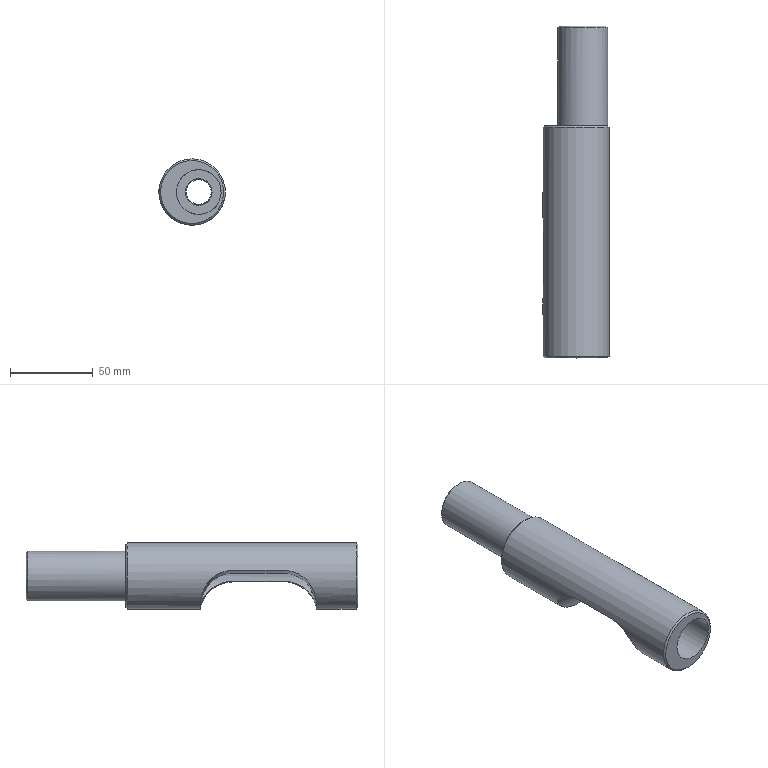Part | NX | features DATUM_CSYS 8, EXTRUDE 8, SKETCH 7, CHAMFER 2 | 1 solid | 19 faces | box 40 x 200 x 40 mm | volume 117689 mm3 | cylinder 8 | plane 8 | cone 3 | commonest cylinder face diameters 40 x3 15 x1 16 x1 27 x1 27.5 x1 30 x1
STEP:
#1=CARTESIAN_POINT('',(12.,40.,0.));
#2=VERTEX_POINT('',#1);
#3=CARTESIAN_POINT('',(4.,40.,0.));
#4=DIRECTION('',(0.,1.,0.));
#5=DIRECTION('',(1.,0.,0.));
#6=AXIS2_PLACEMENT_3D('',#3,#4,#5);
#7=CIRCLE('',#6,8.);
#8=EDGE_CURVE('',#2,#2,#7,.F.);
#9=ORIENTED_EDGE('',*,*,#8,.F.);
#10=EDGE_LOOP('',(#9));
#11=FACE_BOUND('',#10,.T.);
#12=CARTESIAN_POINT('',(4.,-40.,-8.));
#13=VERTEX_POINT('',#12);
#14=CARTESIAN_POINT('',(4.,-40.,0.));
#15=DIRECTION('',(0.,-1.,0.));
#16=DIRECTION('',(0.,0.,-1.));
#17=AXIS2_PLACEMENT_3D('',#14,#15,#16);
#18=CIRCLE('',#17,8.);
#19=EDGE_CURVE('',#13,#13,#18,.F.);
#20=ORIENTED_EDGE('',*,*,#19,.F.);
#21=EDGE_LOOP('',(#20));
#22=FACE_BOUND('',#21,.T.);
#23=CARTESIAN_POINT('',(4.,-192.,0.));
#24=DIRECTION('',(0.,1.,0.));
#25=DIRECTION('',(0.,0.,1.));
#26=AXIS2_PLACEMENT_3D('',#23,#24,#25);
#27=CYLINDRICAL_SURFACE('',#26,8.);
#28=ADVANCED_FACE('',(#11,#22),#27,.F.);
#29=CARTESIAN_POINT('',(0.,-139.,-20.));
#30=VERTEX_POINT('',#29);
#31=CARTESIAN_POINT('',(0.,-139.,0.));
#32=DIRECTION('',(0.,-1.,0.));
#33=DIRECTION('',(0.,0.,-1.));
#34=AXIS2_PLACEMENT_3D('',#31,#32,#33);
#35=CIRCLE('',#34,20.);
#36=EDGE_CURVE('',#30,#30,#35,.F.);
#37=ORIENTED_EDGE('',*,*,#36,.T.);
#38=EDGE_LOOP('',(#37));
#39=FACE_BOUND('',#38,.T.);
#40=CARTESIAN_POINT('',(-19.696,-65.,3.473));
#41=VERTEX_POINT('',#40);
#42=CARTESIAN_POINT('',(-19.696,-95.,3.473));
#43=VERTEX_POINT('',#42);
#44=CARTESIAN_POINT('',(-19.696,-140.,3.473));
#45=DIRECTION('',(0.,1.,0.));
#46=VECTOR('',#45,1000.);
#47=LINE('',#44,#46);
#48=EDGE_CURVE('',#41,#43,#47,.F.);
#49=ORIENTED_EDGE('',*,*,#48,.T.);
#50=CARTESIAN_POINT('',(19.696,-95.,-3.473));
#51=VERTEX_POINT('',#50);
#52=CARTESIAN_POINT('',(-19.696,-95.,3.473));
#53=CARTESIAN_POINT('',(-19.696,-96.79,3.473));
#54=CARTESIAN_POINT('',(-19.786,-100.303,3.009));
#55=CARTESIAN_POINT('',(-20.039,-105.264,0.9372));
#56=CARTESIAN_POINT('',(-19.981,-109.466,-2.426));
#57=CARTESIAN_POINT('',(-19.027,-112.527,-6.766));
#58=CARTESIAN_POINT('',(-16.741,-114.246,-11.36));
#59=CARTESIAN_POINT('',(-11.982,-115.102,-16.706));
#60=CARTESIAN_POINT('',(-3.665,-114.932,-20.648));
#61=CARTESIAN_POINT('',(5.488,-115.101,-19.81));
#62=CARTESIAN_POINT('',(11.786,-114.26,-16.443));
#63=CARTESIAN_POINT('',(15.516,-112.566,-12.928));
#64=CARTESIAN_POINT('',(17.927,-109.514,-9.156));
#65=CARTESIAN_POINT('',(19.146,-105.3,-5.992));
#66=CARTESIAN_POINT('',(19.622,-100.328,-3.944));
#67=CARTESIAN_POINT('',(19.696,-96.794,-3.473));
#68=CARTESIAN_POINT('',(19.696,-95.,-3.473));
#69=B_SPLINE_CURVE_WITH_KNOTS('',3,(#52,#53,#54,#55,#56,#57,#58,#59,#60,#61,#62,#63,#64,#65,#66,#67,#68),.UNSPECIFIED.,.F.,.F.,(4,1,1,1,1,1,1,1,1,1,1,1,1,1,4),(0.,0.005295,0.01059,0.01589,0.02118,0.02648,0.03177,0.04236,0.05295,0.05825,0.06354,0.06884,0.07413,0.07943,0.08472),.UNSPECIFIED.);
#70=EDGE_CURVE('',#43,#51,#69,.T.);
#71=ORIENTED_EDGE('',*,*,#70,.T.);
#72=CARTESIAN_POINT('',(19.696,-65.,-3.473));
#73=VERTEX_POINT('',#72);
#74=CARTESIAN_POINT('',(19.696,-140.,-3.473));
#75=DIRECTION('',(0.,1.,0.));
#76=VECTOR('',#75,1000.);
#77=LINE('',#74,#76);
#78=EDGE_CURVE('',#51,#73,#77,.T.);
#79=ORIENTED_EDGE('',*,*,#78,.T.);
#80=CARTESIAN_POINT('',(19.696,-65.,-3.473));
#81=CARTESIAN_POINT('',(19.696,-63.21,-3.473));
#82=CARTESIAN_POINT('',(19.622,-59.697,-3.94));
#83=CARTESIAN_POINT('',(19.151,-54.736,-5.973));
#84=CARTESIAN_POINT('',(17.946,-50.534,-9.114));
#85=CARTESIAN_POINT('',(15.566,-47.473,-12.866));
#86=CARTESIAN_POINT('',(11.846,-45.754,-16.401));
#87=CARTESIAN_POINT('',(5.545,-44.898,-19.797));
#88=CARTESIAN_POINT('',(-3.618,-45.068,-20.656));
#89=CARTESIAN_POINT('',(-11.933,-44.899,-16.738));
#90=CARTESIAN_POINT('',(-16.699,-45.74,-11.42));
#91=CARTESIAN_POINT('',(-19.002,-47.434,-6.841));
#92=CARTESIAN_POINT('',(-19.978,-50.486,-2.473));
#93=CARTESIAN_POINT('',(-20.04,-54.7,0.9177));
#94=CARTESIAN_POINT('',(-19.787,-59.672,3.005));
#95=CARTESIAN_POINT('',(-19.696,-63.206,3.473));
#96=CARTESIAN_POINT('',(-19.696,-65.,3.473));
#97=B_SPLINE_CURVE_WITH_KNOTS('',3,(#80,#81,#82,#83,#84,#85,#86,#87,#88,#89,#90,#91,#92,#93,#94,#95,#96),.UNSPECIFIED.,.F.,.F.,(4,1,1,1,1,1,1,1,1,1,1,1,1,1,4),(0.,0.005295,0.01059,0.01589,0.02118,0.02648,0.03177,0.04236,0.05295,0.05825,0.06354,0.06884,0.07413,0.07943,0.08472),.UNSPECIFIED.);
#98=EDGE_CURVE('',#73,#41,#97,.T.);
#99=ORIENTED_EDGE('',*,*,#98,.T.);
#100=EDGE_LOOP('',(#49,#71,#79,#99));
#101=FACE_BOUND('',#100,.T.);
#102=CARTESIAN_POINT('',(0.,-1.,-20.));
#103=VERTEX_POINT('',#102);
#104=CARTESIAN_POINT('',(0.,-1.,0.));
#105=DIRECTION('',(0.,-1.,0.));
#106=DIRECTION('',(0.,0.,-1.));
#107=AXIS2_PLACEMENT_3D('',#104,#105,#106);
#108=CIRCLE('',#107,20.);
#109=EDGE_CURVE('',#103,#103,#108,.T.);
#110=ORIENTED_EDGE('',*,*,#109,.T.);
#111=EDGE_LOOP('',(#110));
#112=FACE_BOUND('',#111,.T.);
#113=CARTESIAN_POINT('',(0.,-140.,0.));
#114=DIRECTION('',(0.,1.,0.));
#115=DIRECTION('',(0.,0.,1.));
#116=AXIS2_PLACEMENT_3D('',#113,#114,#115);
#117=CYLINDRICAL_SURFACE('',#116,20.);
#118=ADVANCED_FACE('',(#39,#101,#112),#117,.T.);
#119=CARTESIAN_POINT('',(0.,-140.,-19.));
#120=VERTEX_POINT('',#119);
#121=CARTESIAN_POINT('',(0.,-140.,0.));
#122=DIRECTION('',(0.,-1.,0.));
#123=DIRECTION('',(0.,0.,-1.));
#124=AXIS2_PLACEMENT_3D('',#121,#122,#123);
#125=CIRCLE('',#124,19.);
#126=EDGE_CURVE('',#120,#120,#125,.T.);
#127=ORIENTED_EDGE('',*,*,#126,.T.);
#128=EDGE_LOOP('',(#127));
#129=FACE_BOUND('',#128,.T.);
#130=CARTESIAN_POINT('',(17.5,-140.,0.));
#131=VERTEX_POINT('',#130);
#132=CARTESIAN_POINT('',(4.,-140.,0.));
#133=DIRECTION('',(0.,-1.,0.));
#134=DIRECTION('',(1.,0.,0.));
#135=AXIS2_PLACEMENT_3D('',#132,#133,#134);
#136=CIRCLE('',#135,13.5);
#137=EDGE_CURVE('',#131,#131,#136,.T.);
#138=ORIENTED_EDGE('',*,*,#137,.F.);
#139=EDGE_LOOP('',(#138));
#140=FACE_BOUND('',#139,.T.);
#141=CARTESIAN_POINT('',(0.,-140.,0.));
#142=DIRECTION('',(0.,-1.,0.));
#143=DIRECTION('',(0.,0.,-1.));
#144=AXIS2_PLACEMENT_3D('',#141,#142,#143);
#145=PLANE('',#144);
#146=ADVANCED_FACE('',(#129,#140),#145,.T.);
#147=CARTESIAN_POINT('',(19.,0.,0.));
#148=VERTEX_POINT('',#147);
#149=CARTESIAN_POINT('',(4.,0.,0.));
#150=DIRECTION('',(0.,1.,0.));
#151=DIRECTION('',(1.,0.,0.));
#152=AXIS2_PLACEMENT_3D('',#149,#150,#151);
#153=CIRCLE('',#152,15.);
#154=EDGE_CURVE('',#148,#148,#153,.T.);
#155=ORIENTED_EDGE('',*,*,#154,.F.);
#156=CARTESIAN_POINT('',(0.,0.,0.));
#157=DIRECTION('',(0.,-1.,0.));
#158=DIRECTION('',(0.,0.,-1.));
#159=AXIS2_PLACEMENT_3D('',#156,#157,#158);
#160=CIRCLE('',#159,19.);
#161=EDGE_CURVE('',#148,#148,#160,.F.);
#162=ORIENTED_EDGE('',*,*,#161,.T.);
#163=EDGE_LOOP('',(#155,#162));
#164=FACE_BOUND('',#163,.T.);
#165=CARTESIAN_POINT('',(0.,0.,0.));
#166=DIRECTION('',(0.,-1.,0.));
#167=DIRECTION('',(0.,0.,-1.));
#168=AXIS2_PLACEMENT_3D('',#165,#166,#167);
#169=PLANE('',#168);
#170=ADVANCED_FACE('',(#164),#169,.F.);
#171=CARTESIAN_POINT('',(4.,59.,15.));
#172=VERTEX_POINT('',#171);
#173=CARTESIAN_POINT('',(4.,59.,0.));
#174=DIRECTION('',(0.,1.,0.));
#175=DIRECTION('',(0.,0.,1.));
#176=AXIS2_PLACEMENT_3D('',#173,#174,#175);
#177=CIRCLE('',#176,15.);
#178=EDGE_CURVE('',#172,#172,#177,.F.);
#179=ORIENTED_EDGE('',*,*,#178,.T.);
#180=EDGE_LOOP('',(#179));
#181=FACE_BOUND('',#180,.T.);
#182=ORIENTED_EDGE('',*,*,#154,.T.);
#183=EDGE_LOOP('',(#182));
#184=FACE_BOUND('',#183,.T.);
#185=CARTESIAN_POINT('',(4.,60.,0.));
#186=DIRECTION('',(0.,-1.,0.));
#187=DIRECTION('',(0.,0.,-1.));
#188=AXIS2_PLACEMENT_3D('',#185,#186,#187);
#189=CYLINDRICAL_SURFACE('',#188,15.);
#190=ADVANCED_FACE('',(#181,#184),#189,.T.);
#191=CARTESIAN_POINT('',(4.,60.,14.));
#192=VERTEX_POINT('',#191);
#193=CARTESIAN_POINT('',(4.,60.,0.));
#194=DIRECTION('',(0.,1.,0.));
#195=DIRECTION('',(0.,0.,1.));
#196=AXIS2_PLACEMENT_3D('',#193,#194,#195);
#197=CIRCLE('',#196,14.);
#198=EDGE_CURVE('',#192,#192,#197,.T.);
#199=ORIENTED_EDGE('',*,*,#198,.T.);
#200=EDGE_LOOP('',(#199));
#201=FACE_BOUND('',#200,.T.);
#202=CARTESIAN_POINT('',(11.5,60.,0.));
#203=VERTEX_POINT('',#202);
#204=CARTESIAN_POINT('',(4.,60.,0.));
#205=DIRECTION('',(0.,1.,0.));
#206=DIRECTION('',(1.,0.,0.));
#207=AXIS2_PLACEMENT_3D('',#204,#205,#206);
#208=CIRCLE('',#207,7.5);
#209=EDGE_CURVE('',#203,#203,#208,.T.);
#210=ORIENTED_EDGE('',*,*,#209,.F.);
#211=EDGE_LOOP('',(#210));
#212=FACE_BOUND('',#211,.T.);
#213=CARTESIAN_POINT('',(4.,60.,0.));
#214=DIRECTION('',(0.,1.,0.));
#215=DIRECTION('',(0.,0.,1.));
#216=AXIS2_PLACEMENT_3D('',#213,#214,#215);
#217=PLANE('',#216);
#218=ADVANCED_FACE('',(#201,#212),#217,.T.);
#219=CARTESIAN_POINT('',(11.5,40.,0.));
#220=VERTEX_POINT('',#219);
#221=CARTESIAN_POINT('',(4.,40.,0.));
#222=DIRECTION('',(0.,1.,0.));
#223=DIRECTION('',(1.,0.,0.));
#224=AXIS2_PLACEMENT_3D('',#221,#222,#223);
#225=CIRCLE('',#224,7.5);
#226=EDGE_CURVE('',#220,#220,#225,.F.);
#227=ORIENTED_EDGE('',*,*,#226,.T.);
#228=EDGE_LOOP('',(#227));
#229=FACE_BOUND('',#228,.T.);
#230=ORIENTED_EDGE('',*,*,#209,.T.);
#231=EDGE_LOOP('',(#230));
#232=FACE_BOUND('',#231,.T.);
#233=CARTESIAN_POINT('',(4.,40.,0.));
#234=DIRECTION('',(0.,1.,0.));
#235=DIRECTION('',(0.,0.,1.));
#236=AXIS2_PLACEMENT_3D('',#233,#234,#235);
#237=CYLINDRICAL_SURFACE('',#236,7.5);
#238=ADVANCED_FACE('',(#229,#232),#237,.F.);
#239=ORIENTED_EDGE('',*,*,#8,.T.);
#240=EDGE_LOOP('',(#239));
#241=FACE_BOUND('',#240,.T.);
#242=ORIENTED_EDGE('',*,*,#226,.F.);
#243=EDGE_LOOP('',(#242));
#244=FACE_BOUND('',#243,.T.);
#245=CARTESIAN_POINT('',(4.,40.,0.));
#246=DIRECTION('',(0.,1.,0.));
#247=DIRECTION('',(0.,0.,1.));
#248=AXIS2_PLACEMENT_3D('',#245,#246,#247);
#249=PLANE('',#248);
#250=ADVANCED_FACE('',(#241,#244),#249,.F.);
#251=CARTESIAN_POINT('',(-6.52,-112.,-8.461));
#252=VERTEX_POINT('',#251);
#253=CARTESIAN_POINT('',(10.992,-112.,-11.548));
#254=VERTEX_POINT('',#253);
#255=CARTESIAN_POINT('',(4.,-112.,0.));
#256=DIRECTION('',(0.,-1.,0.));
#257=DIRECTION('',(1.,0.,0.));
#258=AXIS2_PLACEMENT_3D('',#255,#256,#257);
#259=CIRCLE('',#258,13.5);
#260=EDGE_CURVE('',#252,#254,#259,.F.);
#261=ORIENTED_EDGE('',*,*,#260,.T.);
#262=CARTESIAN_POINT('',(10.992,-112.,-11.548));
#263=CARTESIAN_POINT('',(9.672,-112.63,-12.348));
#264=CARTESIAN_POINT('',(6.647,-113.44,-13.545));
#265=CARTESIAN_POINT('',(1.603,-113.771,-13.599));
#266=CARTESIAN_POINT('',(-3.106,-113.442,-11.831));
#267=CARTESIAN_POINT('',(-5.553,-112.63,-9.663));
#268=CARTESIAN_POINT('',(-6.52,-112.,-8.461));
#269=B_SPLINE_CURVE_WITH_KNOTS('',3,(#262,#263,#264,#265,#266,#267,#268),.UNSPECIFIED.,.F.,.F.,(4,1,1,1,4),(0.,0.004926,0.009852,0.01478,0.0197),.UNSPECIFIED.);
#270=EDGE_CURVE('',#254,#252,#269,.T.);
#271=ORIENTED_EDGE('',*,*,#270,.T.);
#272=EDGE_LOOP('',(#261,#271));
#273=FACE_BOUND('',#272,.T.);
#274=ORIENTED_EDGE('',*,*,#137,.T.);
#275=EDGE_LOOP('',(#274));
#276=FACE_BOUND('',#275,.T.);
#277=CARTESIAN_POINT('',(4.,-112.,0.));
#278=DIRECTION('',(0.,-1.,0.));
#279=DIRECTION('',(0.,0.,-1.));
#280=AXIS2_PLACEMENT_3D('',#277,#278,#279);
#281=CYLINDRICAL_SURFACE('',#280,13.5);
#282=ADVANCED_FACE('',(#273,#276),#281,.F.);
#283=CARTESIAN_POINT('',(-6.889,-112.,-8.396));
#284=VERTEX_POINT('',#283);
#285=CARTESIAN_POINT('',(11.361,-112.,-11.614));
#286=VERTEX_POINT('',#285);
#287=CARTESIAN_POINT('',(4.,-112.,0.));
#288=DIRECTION('',(0.,-1.,0.));
#289=DIRECTION('',(1.,0.,0.));
#290=AXIS2_PLACEMENT_3D('',#287,#288,#289);
#291=CIRCLE('',#290,13.75);
#292=EDGE_CURVE('',#284,#286,#291,.F.);
#293=ORIENTED_EDGE('',*,*,#292,.T.);
#294=CARTESIAN_POINT('',(-37.54,-112.,-2.991));
#295=DIRECTION('',(0.9848,0.,-0.1736));
#296=VECTOR('',#295,1000.);
#297=LINE('',#294,#296);
#298=EDGE_CURVE('',#286,#254,#297,.F.);
#299=ORIENTED_EDGE('',*,*,#298,.T.);
#300=ORIENTED_EDGE('',*,*,#260,.F.);
#301=CARTESIAN_POINT('',(-37.54,-112.,-2.991));
#302=DIRECTION('',(0.9848,0.,-0.1736));
#303=VECTOR('',#302,1000.);
#304=LINE('',#301,#303);
#305=EDGE_CURVE('',#252,#284,#304,.F.);
#306=ORIENTED_EDGE('',*,*,#305,.T.);
#307=EDGE_LOOP('',(#293,#299,#300,#306));
#308=FACE_BOUND('',#307,.T.);
#309=CARTESIAN_POINT('',(4.,-112.,0.));
#310=DIRECTION('',(0.,-1.,0.));
#311=DIRECTION('',(0.,0.,-1.));
#312=AXIS2_PLACEMENT_3D('',#309,#310,#311);
#313=PLANE('',#312);
#314=ADVANCED_FACE('',(#308),#313,.F.);
#315=CARTESIAN_POINT('',(17.75,-40.,0.));
#316=VERTEX_POINT('',#315);
#317=CARTESIAN_POINT('',(4.,-40.,0.));
#318=DIRECTION('',(0.,-1.,0.));
#319=DIRECTION('',(1.,0.,0.));
#320=AXIS2_PLACEMENT_3D('',#317,#318,#319);
#321=CIRCLE('',#320,13.75);
#322=EDGE_CURVE('',#316,#316,#321,.F.);
#323=ORIENTED_EDGE('',*,*,#322,.F.);
#324=EDGE_LOOP('',(#323));
#325=FACE_BOUND('',#324,.T.);
#326=ORIENTED_EDGE('',*,*,#19,.T.);
#327=EDGE_LOOP('',(#326));
#328=FACE_BOUND('',#327,.T.);
#329=CARTESIAN_POINT('',(4.,-40.,0.));
#330=DIRECTION('',(0.,-1.,0.));
#331=DIRECTION('',(0.,0.,-1.));
#332=AXIS2_PLACEMENT_3D('',#329,#330,#331);
#333=PLANE('',#332);
#334=ADVANCED_FACE('',(#325,#328),#333,.T.);
#335=ORIENTED_EDGE('',*,*,#292,.F.);
#336=CARTESIAN_POINT('',(-9.644,-95.,1.701));
#337=VERTEX_POINT('',#336);
#338=CARTESIAN_POINT('',(-6.889,-112.,-8.396));
#339=CARTESIAN_POINT('',(-7.902,-111.307,-7.082));
#340=CARTESIAN_POINT('',(-9.269,-109.435,-4.304));
#341=CARTESIAN_POINT('',(-9.814,-105.265,-0.8639));
#342=CARTESIAN_POINT('',(-9.714,-100.303,1.232));
#343=CARTESIAN_POINT('',(-9.644,-96.79,1.701));
#344=CARTESIAN_POINT('',(-9.644,-95.,1.701));
#345=B_SPLINE_CURVE_WITH_KNOTS('',3,(#338,#339,#340,#341,#342,#343,#344),.UNSPECIFIED.,.F.,.F.,(4,1,1,1,4),(0.,0.005308,0.01062,0.01592,0.02123),.UNSPECIFIED.);
#346=EDGE_CURVE('',#284,#337,#345,.T.);
#347=ORIENTED_EDGE('',*,*,#346,.T.);
#348=CARTESIAN_POINT('',(-9.644,-65.,1.701));
#349=VERTEX_POINT('',#348);
#350=CARTESIAN_POINT('',(-9.644,-40.,1.701));
#351=DIRECTION('',(0.,-1.,0.));
#352=VECTOR('',#351,1000.);
#353=LINE('',#350,#352);
#354=EDGE_CURVE('',#337,#349,#353,.F.);
#355=ORIENTED_EDGE('',*,*,#354,.T.);
#356=CARTESIAN_POINT('',(17.403,-65.,-3.069));
#357=VERTEX_POINT('',#356);
#358=CARTESIAN_POINT('',(-9.644,-65.,1.701));
#359=CARTESIAN_POINT('',(-9.644,-62.343,1.701));
#360=CARTESIAN_POINT('',(-9.789,-58.41,0.9118));
#361=CARTESIAN_POINT('',(-9.718,-53.802,-1.612));
#362=CARTESIAN_POINT('',(-9.201,-50.797,-4.218));
#363=CARTESIAN_POINT('',(-7.863,-48.525,-7.249));
#364=CARTESIAN_POINT('',(-4.731,-46.627,-11.161));
#365=CARTESIAN_POINT('',(1.429,-45.996,-14.333));
#366=CARTESIAN_POINT('',(8.288,-46.608,-13.505));
#367=CARTESIAN_POINT('',(12.6,-48.479,-10.926));
#368=CARTESIAN_POINT('',(15.696,-51.488,-7.728));
#369=CARTESIAN_POINT('',(17.234,-57.079,-4.101));
#370=CARTESIAN_POINT('',(17.403,-62.337,-3.069));
#371=CARTESIAN_POINT('',(17.403,-65.,-3.069));
#372=B_SPLINE_CURVE_WITH_KNOTS('',3,(#358,#359,#360,#361,#362,#363,#364,#365,#366,#367,#368,#369,#370,#371),.UNSPECIFIED.,.F.,.F.,(4,1,1,1,1,1,1,1,1,1,1,4),(0.,0.007848,0.01177,0.0157,0.01962,0.02354,0.03139,0.03924,0.04316,0.04709,0.05494,0.06279),.UNSPECIFIED.);
#373=EDGE_CURVE('',#349,#357,#372,.T.);
#374=ORIENTED_EDGE('',*,*,#373,.T.);
#375=CARTESIAN_POINT('',(17.403,-95.,-3.069));
#376=VERTEX_POINT('',#375);
#377=CARTESIAN_POINT('',(17.403,-40.,-3.069));
#378=DIRECTION('',(0.,-1.,0.));
#379=VECTOR('',#378,1000.);
#380=LINE('',#377,#379);
#381=EDGE_CURVE('',#357,#376,#380,.T.);
#382=ORIENTED_EDGE('',*,*,#381,.T.);
#383=CARTESIAN_POINT('',(17.403,-95.,-3.069));
#384=CARTESIAN_POINT('',(17.403,-96.791,-3.069));
#385=CARTESIAN_POINT('',(17.31,-100.297,-3.531));
#386=CARTESIAN_POINT('',(16.685,-105.256,-5.533));
#387=CARTESIAN_POINT('',(15.013,-109.414,-8.564));
#388=CARTESIAN_POINT('',(12.764,-111.306,-10.724));
#389=CARTESIAN_POINT('',(11.361,-112.,-11.614));
#390=B_SPLINE_CURVE_WITH_KNOTS('',3,(#383,#384,#385,#386,#387,#388,#389),.UNSPECIFIED.,.F.,.F.,(4,1,1,1,4),(0.,0.005289,0.01058,0.01587,0.02116),.UNSPECIFIED.);
#391=EDGE_CURVE('',#376,#286,#390,.T.);
#392=ORIENTED_EDGE('',*,*,#391,.T.);
#393=EDGE_LOOP('',(#335,#347,#355,#374,#382,#392));
#394=FACE_BOUND('',#393,.T.);
#395=ORIENTED_EDGE('',*,*,#322,.T.);
#396=EDGE_LOOP('',(#395));
#397=FACE_BOUND('',#396,.T.);
#398=CARTESIAN_POINT('',(4.,-40.,0.));
#399=DIRECTION('',(0.,-1.,0.));
#400=DIRECTION('',(0.,0.,-1.));
#401=AXIS2_PLACEMENT_3D('',#398,#399,#400);
#402=CYLINDRICAL_SURFACE('',#401,13.75);
#403=ADVANCED_FACE('',(#394,#397),#402,.F.);
#404=ORIENTED_EDGE('',*,*,#161,.F.);
#405=EDGE_LOOP('',(#404));
#406=FACE_BOUND('',#405,.T.);
#407=ORIENTED_EDGE('',*,*,#109,.F.);
#408=EDGE_LOOP('',(#407));
#409=FACE_BOUND('',#408,.T.);
#410=CARTESIAN_POINT('',(0.,-1.,0.));
#411=DIRECTION('',(0.,-1.,0.));
#412=DIRECTION('',(0.,0.,-1.));
#413=AXIS2_PLACEMENT_3D('',#410,#411,#412);
#414=CONICAL_SURFACE('',#413,20.,0.7854);
#415=ADVANCED_FACE('',(#406,#409),#414,.T.);
#416=ORIENTED_EDGE('',*,*,#178,.F.);
#417=EDGE_LOOP('',(#416));
#418=FACE_BOUND('',#417,.T.);
#419=ORIENTED_EDGE('',*,*,#198,.F.);
#420=EDGE_LOOP('',(#419));
#421=FACE_BOUND('',#420,.T.);
#422=CARTESIAN_POINT('',(4.,60.,0.));
#423=DIRECTION('',(0.,-1.,0.));
#424=DIRECTION('',(0.,0.,-1.));
#425=AXIS2_PLACEMENT_3D('',#422,#423,#424);
#426=CONICAL_SURFACE('',#425,14.,0.7854);
#427=ADVANCED_FACE('',(#418,#421),#426,.T.);
#428=CARTESIAN_POINT('',(-35.897,-95.,6.33));
#429=DIRECTION('',(0.9848,0.,-0.1736));
#430=VECTOR('',#429,1000.);
#431=LINE('',#428,#430);
#432=EDGE_CURVE('',#51,#376,#431,.F.);
#433=ORIENTED_EDGE('',*,*,#432,.T.);
#434=ORIENTED_EDGE('',*,*,#381,.F.);
#435=CARTESIAN_POINT('',(-35.897,-65.,6.33));
#436=DIRECTION('',(0.9848,0.,-0.1736));
#437=VECTOR('',#436,1000.);
#438=LINE('',#435,#437);
#439=EDGE_CURVE('',#73,#357,#438,.F.);
#440=ORIENTED_EDGE('',*,*,#439,.F.);
#441=ORIENTED_EDGE('',*,*,#78,.F.);
#442=EDGE_LOOP('',(#433,#434,#440,#441));
#443=FACE_BOUND('',#442,.T.);
#444=CARTESIAN_POINT('',(-35.897,-65.,6.33));
#445=DIRECTION('',(0.1736,0.,0.9848));
#446=DIRECTION('',(0.9848,0.,-0.1736));
#447=AXIS2_PLACEMENT_3D('',#444,#445,#446);
#448=PLANE('',#447);
#449=ADVANCED_FACE('',(#443),#448,.F.);
#450=CARTESIAN_POINT('',(-35.897,-65.,6.33));
#451=DIRECTION('',(0.9848,0.,-0.1736));
#452=VECTOR('',#451,1000.);
#453=LINE('',#450,#452);
#454=EDGE_CURVE('',#349,#41,#453,.F.);
#455=ORIENTED_EDGE('',*,*,#454,.F.);
#456=ORIENTED_EDGE('',*,*,#354,.F.);
#457=CARTESIAN_POINT('',(-35.897,-95.,6.33));
#458=DIRECTION('',(0.9848,0.,-0.1736));
#459=VECTOR('',#458,1000.);
#460=LINE('',#457,#459);
#461=EDGE_CURVE('',#337,#43,#460,.F.);
#462=ORIENTED_EDGE('',*,*,#461,.T.);
#463=ORIENTED_EDGE('',*,*,#48,.F.);
#464=EDGE_LOOP('',(#455,#456,#462,#463));
#465=FACE_BOUND('',#464,.T.);
#466=CARTESIAN_POINT('',(-35.897,-65.,6.33));
#467=DIRECTION('',(0.1736,0.,0.9848));
#468=DIRECTION('',(0.9848,0.,-0.1736));
#469=AXIS2_PLACEMENT_3D('',#466,#467,#468);
#470=PLANE('',#469);
#471=ADVANCED_FACE('',(#465),#470,.F.);
#472=ORIENTED_EDGE('',*,*,#461,.F.);
#473=ORIENTED_EDGE('',*,*,#346,.F.);
#474=ORIENTED_EDGE('',*,*,#305,.F.);
#475=ORIENTED_EDGE('',*,*,#270,.F.);
#476=ORIENTED_EDGE('',*,*,#298,.F.);
#477=ORIENTED_EDGE('',*,*,#391,.F.);
#478=ORIENTED_EDGE('',*,*,#432,.F.);
#479=ORIENTED_EDGE('',*,*,#70,.F.);
#480=EDGE_LOOP('',(#472,#473,#474,#475,#476,#477,#478,#479));
#481=FACE_BOUND('',#480,.T.);
#482=CARTESIAN_POINT('',(-39.37,-95.,-13.367));
#483=DIRECTION('',(0.9848,0.,-0.1736));
#484=DIRECTION('',(-0.1736,0.,-0.9848));
#485=AXIS2_PLACEMENT_3D('',#482,#483,#484);
#486=CYLINDRICAL_SURFACE('',#485,20.);
#487=ADVANCED_FACE('',(#481),#486,.F.);
#488=ORIENTED_EDGE('',*,*,#439,.T.);
#489=ORIENTED_EDGE('',*,*,#373,.F.);
#490=ORIENTED_EDGE('',*,*,#454,.T.);
#491=ORIENTED_EDGE('',*,*,#98,.F.);
#492=EDGE_LOOP('',(#488,#489,#490,#491));
#493=FACE_BOUND('',#492,.T.);
#494=CARTESIAN_POINT('',(-39.37,-65.,-13.367));
#495=DIRECTION('',(0.9848,0.,-0.1736));
#496=DIRECTION('',(-0.1736,0.,-0.9848));
#497=AXIS2_PLACEMENT_3D('',#494,#495,#496);
#498=CYLINDRICAL_SURFACE('',#497,20.);
#499=ADVANCED_FACE('',(#493),#498,.F.);
#500=ORIENTED_EDGE('',*,*,#36,.F.);
#501=EDGE_LOOP('',(#500));
#502=FACE_BOUND('',#501,.T.);
#503=ORIENTED_EDGE('',*,*,#126,.F.);
#504=EDGE_LOOP('',(#503));
#505=FACE_BOUND('',#504,.T.);
#506=CARTESIAN_POINT('',(0.,-140.,0.));
#507=DIRECTION('',(0.,1.,0.));
#508=DIRECTION('',(0.,0.,1.));
#509=AXIS2_PLACEMENT_3D('',#506,#507,#508);
#510=CONICAL_SURFACE('',#509,19.,0.7854);
#511=ADVANCED_FACE('',(#502,#505),#510,.T.);
#512=CLOSED_SHELL('',(#28,#118,#146,#170,#190,#218,#238,#250,#282,#314,#334,#403,#415,#427,#449,#471,#487,#499,#511));
#513=MANIFOLD_SOLID_BREP('',#512);
#514=(LENGTH_UNIT()NAMED_UNIT(*)SI_UNIT(.MILLI.,.METRE.));
#515=UNCERTAINTY_MEASURE_WITH_UNIT(LENGTH_MEASURE(0.0508),#514,'','');
#516=(NAMED_UNIT(*)PLANE_ANGLE_UNIT()SI_UNIT($,.RADIAN.));
#517=(NAMED_UNIT(*)SI_UNIT($,.STERADIAN.)SOLID_ANGLE_UNIT());
#518=(GEOMETRIC_REPRESENTATION_CONTEXT(3)GLOBAL_UNCERTAINTY_ASSIGNED_CONTEXT((#515))GLOBAL_UNIT_ASSIGNED_CONTEXT((#514,#516,#517))REPRESENTATION_CONTEXT('',''));
#519=ADVANCED_BREP_SHAPE_REPRESENTATION('',(#513),#518);